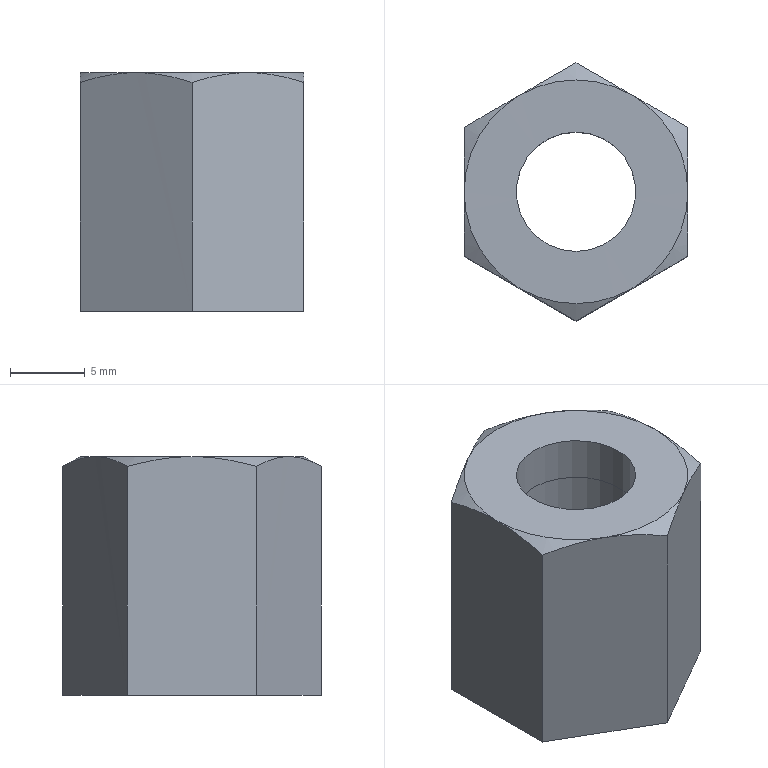Part | STEP file | 1-11.2 | 2 solids | 21 faces | box 15 x 17.321 x 16 mm | volume 1681 mm3 | plane 11 | cone 6 | cylinder 4 | commonest cylinder face diameters 8 x2 12 x2